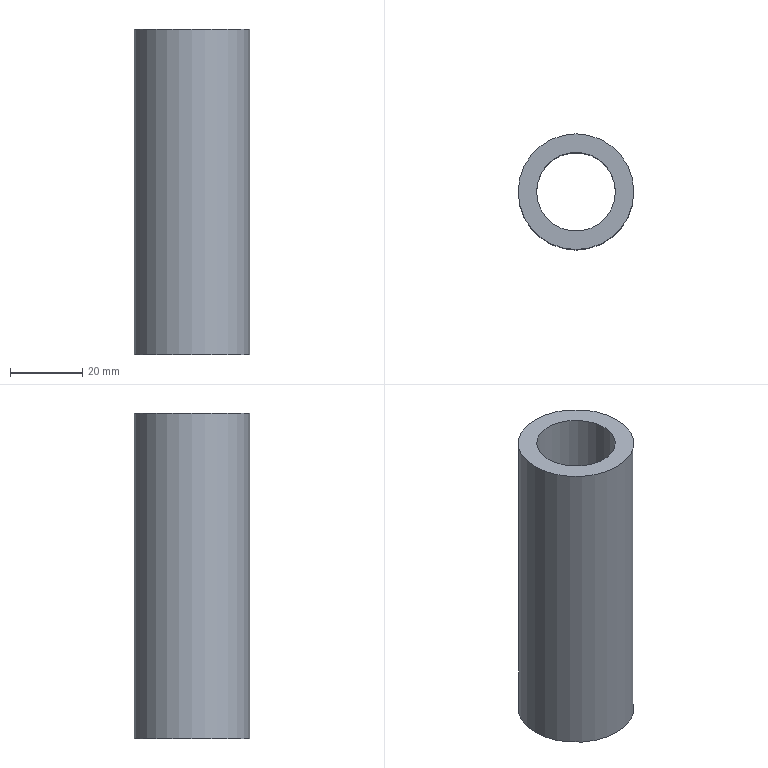Part | NX | features solid 2 | 1 solid | 4 faces | box 32 x 32 x 90 mm | volume 38790 mm3 | plane 2 | cylinder 2 | commonest cylinder face diameters 21.8 x1 32 x1
STEP:
#1=CARTESIAN_POINT('',(-424.,575.,145.));
#2=VERTEX_POINT('',#1);
#3=CARTESIAN_POINT('',(-440.,575.,145.));
#4=DIRECTION('',(0.,0.,1.));
#5=DIRECTION('',(1.,0.,0.));
#6=AXIS2_PLACEMENT_3D('',#3,#4,#5);
#7=CIRCLE('',#6,16.);
#8=EDGE_CURVE('',#2,#2,#7,.T.);
#9=ORIENTED_EDGE('',*,*,#8,.F.);
#10=EDGE_LOOP('',(#9));
#11=FACE_BOUND('',#10,.T.);
#12=CARTESIAN_POINT('',(-429.1,575.,145.));
#13=VERTEX_POINT('',#12);
#14=CARTESIAN_POINT('',(-440.,575.,145.));
#15=DIRECTION('',(0.,0.,1.));
#16=DIRECTION('',(1.,0.,0.));
#17=AXIS2_PLACEMENT_3D('',#14,#15,#16);
#18=CIRCLE('',#17,10.9);
#19=EDGE_CURVE('',#13,#13,#18,.F.);
#20=ORIENTED_EDGE('',*,*,#19,.F.);
#21=EDGE_LOOP('',(#20));
#22=FACE_BOUND('',#21,.T.);
#23=CARTESIAN_POINT('',(-440.,575.,145.));
#24=DIRECTION('',(0.,0.,-1.));
#25=DIRECTION('',(0.,1.,0.));
#26=AXIS2_PLACEMENT_3D('',#23,#24,#25);
#27=PLANE('',#26);
#28=ADVANCED_FACE('',(#11,#22),#27,.T.);
#29=CARTESIAN_POINT('',(-424.,575.,235.));
#30=VERTEX_POINT('',#29);
#31=CARTESIAN_POINT('',(-440.,575.,235.));
#32=DIRECTION('',(0.,0.,1.));
#33=DIRECTION('',(1.,0.,0.));
#34=AXIS2_PLACEMENT_3D('',#31,#32,#33);
#35=CIRCLE('',#34,16.);
#36=EDGE_CURVE('',#30,#30,#35,.T.);
#37=ORIENTED_EDGE('',*,*,#36,.F.);
#38=EDGE_LOOP('',(#37));
#39=FACE_BOUND('',#38,.T.);
#40=ORIENTED_EDGE('',*,*,#8,.T.);
#41=EDGE_LOOP('',(#40));
#42=FACE_BOUND('',#41,.T.);
#43=CARTESIAN_POINT('',(-440.,575.,125.));
#44=DIRECTION('',(0.,0.,1.));
#45=DIRECTION('',(0.,-1.,0.));
#46=AXIS2_PLACEMENT_3D('',#43,#44,#45);
#47=CYLINDRICAL_SURFACE('',#46,16.);
#48=ADVANCED_FACE('',(#39,#42),#47,.T.);
#49=ORIENTED_EDGE('',*,*,#36,.T.);
#50=EDGE_LOOP('',(#49));
#51=FACE_BOUND('',#50,.T.);
#52=CARTESIAN_POINT('',(-429.1,575.,235.));
#53=VERTEX_POINT('',#52);
#54=CARTESIAN_POINT('',(-440.,575.,235.));
#55=DIRECTION('',(0.,0.,1.));
#56=DIRECTION('',(1.,0.,0.));
#57=AXIS2_PLACEMENT_3D('',#54,#55,#56);
#58=CIRCLE('',#57,10.9);
#59=EDGE_CURVE('',#53,#53,#58,.T.);
#60=ORIENTED_EDGE('',*,*,#59,.F.);
#61=EDGE_LOOP('',(#60));
#62=FACE_BOUND('',#61,.T.);
#63=CARTESIAN_POINT('',(-440.,575.,235.));
#64=DIRECTION('',(0.,0.,-1.));
#65=DIRECTION('',(0.,1.,0.));
#66=AXIS2_PLACEMENT_3D('',#63,#64,#65);
#67=PLANE('',#66);
#68=ADVANCED_FACE('',(#51,#62),#67,.F.);
#69=ORIENTED_EDGE('',*,*,#19,.T.);
#70=EDGE_LOOP('',(#69));
#71=FACE_BOUND('',#70,.T.);
#72=ORIENTED_EDGE('',*,*,#59,.T.);
#73=EDGE_LOOP('',(#72));
#74=FACE_BOUND('',#73,.T.);
#75=CARTESIAN_POINT('',(-440.,575.,125.));
#76=DIRECTION('',(0.,0.,1.));
#77=DIRECTION('',(0.,-1.,0.));
#78=AXIS2_PLACEMENT_3D('',#75,#76,#77);
#79=CYLINDRICAL_SURFACE('',#78,10.9);
#80=ADVANCED_FACE('',(#71,#74),#79,.F.);
#81=CLOSED_SHELL('',(#28,#48,#68,#80));
#82=MANIFOLD_SOLID_BREP('',#81);
#83=(LENGTH_UNIT()NAMED_UNIT(*)SI_UNIT(.MILLI.,.METRE.));
#84=UNCERTAINTY_MEASURE_WITH_UNIT(LENGTH_MEASURE(0.00001),#83,'','');
#85=(NAMED_UNIT(*)PLANE_ANGLE_UNIT()SI_UNIT($,.RADIAN.));
#86=(NAMED_UNIT(*)SI_UNIT($,.STERADIAN.)SOLID_ANGLE_UNIT());
#87=(GEOMETRIC_REPRESENTATION_CONTEXT(3)GLOBAL_UNCERTAINTY_ASSIGNED_CONTEXT((#84))GLOBAL_UNIT_ASSIGNED_CONTEXT((#83,#85,#86))REPRESENTATION_CONTEXT('',''));
#88=ADVANCED_BREP_SHAPE_REPRESENTATION('',(#82),#87);